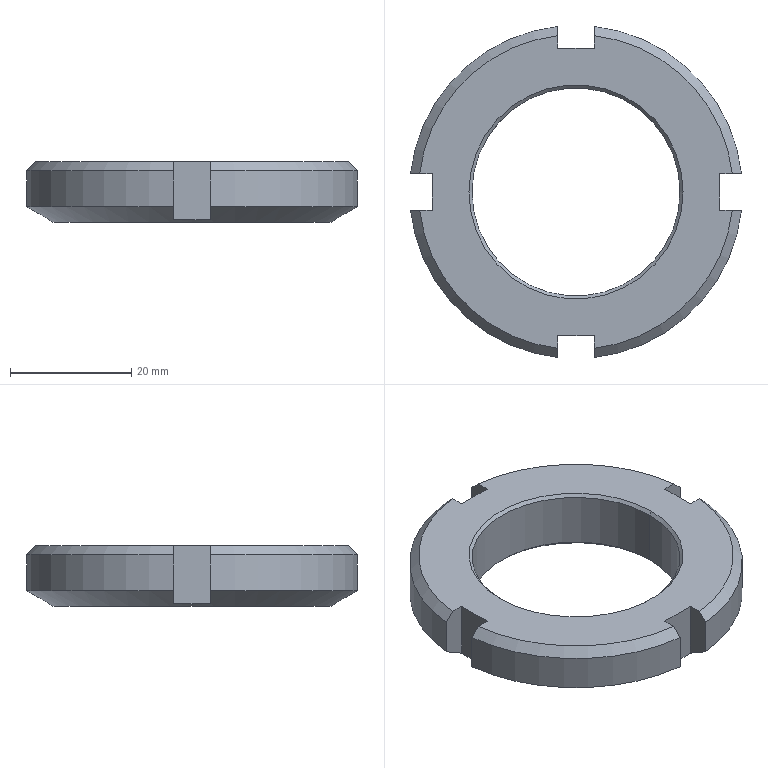Part | SolidWorks | features Chamfer 3, CirPattern 1, Cut 1, Extrusion 1 | 1 solid | 30 faces | box 54.672 x 54.672 x 10 mm | volume 12577 mm3 | plane 14 | cone 10 | cylinder 6 | commonest cylinder face diameters 55 x4 34.376 x2
STEP:
#1=CARTESIAN_POINT('',(-17.188,0.,9.5));
#2=VERTEX_POINT('',#1);
#3=CARTESIAN_POINT('',(17.188,0.,9.5));
#4=VERTEX_POINT('',#3);
#5=CARTESIAN_POINT('',(0.,0.,9.5));
#6=DIRECTION('',(0.,0.,1.));
#7=DIRECTION('',(1.,0.,0.));
#8=AXIS2_PLACEMENT_3D('',#5,#6,#7);
#9=CIRCLE('',#8,17.188);
#10=EDGE_CURVE('',#2,#4,#9,.T.);
#11=ORIENTED_EDGE('',*,*,#10,.F.);
#12=CARTESIAN_POINT('',(-17.688,0.,10.));
#13=VERTEX_POINT('',#12);
#14=CARTESIAN_POINT('',(-17.188,0.,9.5));
#15=DIRECTION('',(-0.7071,0.,0.7071));
#16=VECTOR('',#15,1000.);
#17=LINE('',#14,#16);
#18=EDGE_CURVE('',#2,#13,#17,.T.);
#19=ORIENTED_EDGE('',*,*,#18,.T.);
#20=CARTESIAN_POINT('',(17.688,0.,10.));
#21=VERTEX_POINT('',#20);
#22=CARTESIAN_POINT('',(0.,0.,10.));
#23=DIRECTION('',(0.,0.,-1.));
#24=DIRECTION('',(1.,0.,0.));
#25=AXIS2_PLACEMENT_3D('',#22,#23,#24);
#26=CIRCLE('',#25,17.688);
#27=EDGE_CURVE('',#21,#13,#26,.T.);
#28=ORIENTED_EDGE('',*,*,#27,.F.);
#29=CARTESIAN_POINT('',(17.188,0.,9.5));
#30=DIRECTION('',(0.7071,0.,0.7071));
#31=VECTOR('',#30,1000.);
#32=LINE('',#29,#31);
#33=EDGE_CURVE('',#4,#21,#32,.T.);
#34=ORIENTED_EDGE('',*,*,#33,.F.);
#35=EDGE_LOOP('',(#11,#19,#28,#34));
#36=FACE_OUTER_BOUND('',#35,.T.);
#37=CARTESIAN_POINT('',(0.,0.,9.5));
#38=DIRECTION('',(0.,0.,1.));
#39=DIRECTION('',(1.,0.,0.));
#40=AXIS2_PLACEMENT_3D('',#37,#38,#39);
#41=CONICAL_SURFACE('',#40,17.188,0.7854);
#42=ADVANCED_FACE('',(#36),#41,.F.);
#43=CARTESIAN_POINT('',(17.188,0.,0.5));
#44=VERTEX_POINT('',#43);
#45=CARTESIAN_POINT('',(-17.188,0.,0.5));
#46=VERTEX_POINT('',#45);
#47=CARTESIAN_POINT('',(0.,0.,0.5));
#48=DIRECTION('',(0.,0.,-1.));
#49=DIRECTION('',(1.,0.,0.));
#50=AXIS2_PLACEMENT_3D('',#47,#48,#49);
#51=CIRCLE('',#50,17.188);
#52=EDGE_CURVE('',#44,#46,#51,.T.);
#53=ORIENTED_EDGE('',*,*,#52,.F.);
#54=CARTESIAN_POINT('',(17.688,0.,0.));
#55=VERTEX_POINT('',#54);
#56=CARTESIAN_POINT('',(17.688,0.,0.));
#57=DIRECTION('',(0.7071,0.,-0.7071));
#58=VECTOR('',#57,1000.);
#59=LINE('',#56,#58);
#60=EDGE_CURVE('',#44,#55,#59,.T.);
#61=ORIENTED_EDGE('',*,*,#60,.T.);
#62=CARTESIAN_POINT('',(-17.688,0.,0.));
#63=VERTEX_POINT('',#62);
#64=CARTESIAN_POINT('',(0.,0.,0.));
#65=DIRECTION('',(0.,0.,1.));
#66=DIRECTION('',(1.,0.,0.));
#67=AXIS2_PLACEMENT_3D('',#64,#65,#66);
#68=CIRCLE('',#67,17.688);
#69=EDGE_CURVE('',#63,#55,#68,.T.);
#70=ORIENTED_EDGE('',*,*,#69,.F.);
#71=CARTESIAN_POINT('',(-17.688,0.,0.));
#72=DIRECTION('',(-0.7071,0.,-0.7071));
#73=VECTOR('',#72,1000.);
#74=LINE('',#71,#73);
#75=EDGE_CURVE('',#46,#63,#74,.T.);
#76=ORIENTED_EDGE('',*,*,#75,.F.);
#77=EDGE_LOOP('',(#53,#61,#70,#76));
#78=FACE_OUTER_BOUND('',#77,.T.);
#79=CARTESIAN_POINT('',(0.,0.,0.));
#80=DIRECTION('',(0.,0.,-1.));
#81=DIRECTION('',(-1.,0.,0.));
#82=AXIS2_PLACEMENT_3D('',#79,#80,#81);
#83=CONICAL_SURFACE('',#82,17.688,0.7854);
#84=ADVANCED_FACE('',(#78),#83,.F.);
#85=CARTESIAN_POINT('',(-23.,0.,0.));
#86=VERTEX_POINT('',#85);
#87=CARTESIAN_POINT('',(23.,0.,0.));
#88=VERTEX_POINT('',#87);
#89=CARTESIAN_POINT('',(0.,0.,0.));
#90=DIRECTION('',(0.,0.,-1.));
#91=DIRECTION('',(1.,0.,0.));
#92=AXIS2_PLACEMENT_3D('',#89,#90,#91);
#93=CIRCLE('',#92,23.);
#94=EDGE_CURVE('',#86,#88,#93,.T.);
#95=ORIENTED_EDGE('',*,*,#94,.F.);
#96=CARTESIAN_POINT('',(-23.736,0.,0.4249));
#97=VERTEX_POINT('',#96);
#98=CARTESIAN_POINT('',(-27.5,0.,2.598));
#99=DIRECTION('',(-0.866,0.,0.5));
#100=VECTOR('',#99,1000.);
#101=LINE('',#98,#100);
#102=EDGE_CURVE('',#86,#97,#101,.T.);
#103=ORIENTED_EDGE('',*,*,#102,.T.);
#104=CARTESIAN_POINT('',(-23.736,3.,0.5339));
#105=VERTEX_POINT('',#104);
#106=CARTESIAN_POINT('',(-23.736,3.,0.5339));
#107=CARTESIAN_POINT('',(-23.736,2.004,0.4617));
#108=CARTESIAN_POINT('',(-23.736,1.004,0.4249));
#109=CARTESIAN_POINT('',(-23.736,0.,0.4249));
#110=B_SPLINE_CURVE_WITH_KNOTS('',3,(#106,#107,#108,#109),.UNSPECIFIED.,.F.,.F.,(4,4),(0.008011,0.01101),.UNSPECIFIED.);
#111=EDGE_CURVE('',#105,#97,#110,.T.);
#112=ORIENTED_EDGE('',*,*,#111,.F.);
#113=CARTESIAN_POINT('',(-27.336,3.,2.598));
#114=VERTEX_POINT('',#113);
#115=CARTESIAN_POINT('',(-27.336,3.,2.598));
#116=CARTESIAN_POINT('',(-26.136,3.,1.91));
#117=CARTESIAN_POINT('',(-24.936,3.,1.221));
#118=CARTESIAN_POINT('',(-23.736,3.,0.5339));
#119=B_SPLINE_CURVE_WITH_KNOTS('',3,(#115,#116,#117,#118),.UNSPECIFIED.,.F.,.F.,(4,4),(0.007772,0.01192),.UNSPECIFIED.);
#120=EDGE_CURVE('',#114,#105,#119,.T.);
#121=ORIENTED_EDGE('',*,*,#120,.F.);
#122=CARTESIAN_POINT('',(-3.,27.336,2.598));
#123=VERTEX_POINT('',#122);
#124=CARTESIAN_POINT('',(0.,0.,2.598));
#125=DIRECTION('',(0.,0.,1.));
#126=DIRECTION('',(1.,0.,0.));
#127=AXIS2_PLACEMENT_3D('',#124,#125,#126);
#128=CIRCLE('',#127,27.5);
#129=EDGE_CURVE('',#123,#114,#128,.T.);
#130=ORIENTED_EDGE('',*,*,#129,.F.);
#131=CARTESIAN_POINT('',(-3.,23.736,0.5339));
#132=VERTEX_POINT('',#131);
#133=CARTESIAN_POINT('',(-3.,23.736,0.5339));
#134=CARTESIAN_POINT('',(-3.,24.936,1.221));
#135=CARTESIAN_POINT('',(-3.,26.136,1.91));
#136=CARTESIAN_POINT('',(-3.,27.336,2.598));
#137=B_SPLINE_CURVE_WITH_KNOTS('',3,(#133,#134,#135,#136),.UNSPECIFIED.,.F.,.F.,(4,4),(0.008037,0.01219),.UNSPECIFIED.);
#138=EDGE_CURVE('',#132,#123,#137,.T.);
#139=ORIENTED_EDGE('',*,*,#138,.F.);
#140=CARTESIAN_POINT('',(3.,23.736,0.5339));
#141=VERTEX_POINT('',#140);
#142=CARTESIAN_POINT('',(3.,23.736,0.5339));
#143=CARTESIAN_POINT('',(2.007,23.736,0.462));
#144=CARTESIAN_POINT('',(1.01,23.736,0.4251));
#145=CARTESIAN_POINT('',(-0.9903,23.736,0.4246));
#146=CARTESIAN_POINT('',(-1.998,23.736,0.4613));
#147=CARTESIAN_POINT('',(-3.,23.736,0.5339));
#148=B_SPLINE_CURVE_WITH_KNOTS('',3,(#142,#143,#144,#145,#146,#147),.UNSPECIFIED.,.F.,.F.,(4,2,4),(0.008011,0.011,0.01398),.UNSPECIFIED.);
#149=EDGE_CURVE('',#141,#132,#148,.T.);
#150=ORIENTED_EDGE('',*,*,#149,.F.);
#151=CARTESIAN_POINT('',(3.,27.336,2.598));
#152=VERTEX_POINT('',#151);
#153=CARTESIAN_POINT('',(3.,27.336,2.598));
#154=CARTESIAN_POINT('',(3.,26.136,1.91));
#155=CARTESIAN_POINT('',(3.,24.936,1.221));
#156=CARTESIAN_POINT('',(3.,23.736,0.5339));
#157=B_SPLINE_CURVE_WITH_KNOTS('',3,(#153,#154,#155,#156),.UNSPECIFIED.,.F.,.F.,(4,4),(0.004783,0.008933),.UNSPECIFIED.);
#158=EDGE_CURVE('',#152,#141,#157,.T.);
#159=ORIENTED_EDGE('',*,*,#158,.F.);
#160=CARTESIAN_POINT('',(27.336,3.,2.598));
#161=VERTEX_POINT('',#160);
#162=CARTESIAN_POINT('',(0.,0.,2.598));
#163=DIRECTION('',(0.,0.,1.));
#164=DIRECTION('',(1.,0.,0.));
#165=AXIS2_PLACEMENT_3D('',#162,#163,#164);
#166=CIRCLE('',#165,27.5);
#167=EDGE_CURVE('',#161,#152,#166,.T.);
#168=ORIENTED_EDGE('',*,*,#167,.F.);
#169=CARTESIAN_POINT('',(23.736,3.,0.5339));
#170=VERTEX_POINT('',#169);
#171=CARTESIAN_POINT('',(23.736,3.,0.5339));
#172=CARTESIAN_POINT('',(24.936,3.,1.221));
#173=CARTESIAN_POINT('',(26.136,3.,1.91));
#174=CARTESIAN_POINT('',(27.336,3.,2.598));
#175=B_SPLINE_CURVE_WITH_KNOTS('',3,(#171,#172,#173,#174),.UNSPECIFIED.,.F.,.F.,(4,4),(0.008037,0.01219),.UNSPECIFIED.);
#176=EDGE_CURVE('',#170,#161,#175,.T.);
#177=ORIENTED_EDGE('',*,*,#176,.F.);
#178=CARTESIAN_POINT('',(23.736,0.,0.4249));
#179=VERTEX_POINT('',#178);
#180=CARTESIAN_POINT('',(23.736,0.,0.4249));
#181=CARTESIAN_POINT('',(23.736,1.004,0.4249));
#182=CARTESIAN_POINT('',(23.736,2.004,0.4617));
#183=CARTESIAN_POINT('',(23.736,3.,0.5339));
#184=B_SPLINE_CURVE_WITH_KNOTS('',3,(#180,#181,#182,#183),.UNSPECIFIED.,.F.,.F.,(4,4),(0.01546,0.01847),.UNSPECIFIED.);
#185=EDGE_CURVE('',#179,#170,#184,.T.);
#186=ORIENTED_EDGE('',*,*,#185,.F.);
#187=CARTESIAN_POINT('',(27.5,0.,2.598));
#188=DIRECTION('',(0.866,0.,0.5));
#189=VECTOR('',#188,1000.);
#190=LINE('',#187,#189);
#191=EDGE_CURVE('',#88,#179,#190,.T.);
#192=ORIENTED_EDGE('',*,*,#191,.F.);
#193=EDGE_LOOP('',(#95,#103,#112,#121,#130,#139,#150,#159,#168,#177,#186,#192));
#194=FACE_OUTER_BOUND('',#193,.T.);
#195=CARTESIAN_POINT('',(0.,0.,2.598));
#196=DIRECTION('',(0.,0.,1.));
#197=DIRECTION('',(1.,0.,0.));
#198=AXIS2_PLACEMENT_3D('',#195,#196,#197);
#199=CONICAL_SURFACE('',#198,27.5,1.047);
#200=ADVANCED_FACE('',(#194),#199,.T.);
#201=ORIENTED_EDGE('',*,*,#10,.T.);
#202=CARTESIAN_POINT('',(17.188,0.,10.));
#203=DIRECTION('',(0.,0.,-1.));
#204=VECTOR('',#203,1000.);
#205=LINE('',#202,#204);
#206=EDGE_CURVE('',#4,#44,#205,.T.);
#207=ORIENTED_EDGE('',*,*,#206,.T.);
#208=ORIENTED_EDGE('',*,*,#52,.T.);
#209=CARTESIAN_POINT('',(-17.188,0.,10.));
#210=DIRECTION('',(0.,0.,-1.));
#211=VECTOR('',#210,1000.);
#212=LINE('',#209,#211);
#213=EDGE_CURVE('',#2,#46,#212,.T.);
#214=ORIENTED_EDGE('',*,*,#213,.F.);
#215=EDGE_LOOP('',(#201,#207,#208,#214));
#216=FACE_OUTER_BOUND('',#215,.T.);
#217=CARTESIAN_POINT('',(0.,0.,10.));
#218=DIRECTION('',(0.,0.,-1.));
#219=DIRECTION('',(-1.,0.,0.));
#220=AXIS2_PLACEMENT_3D('',#217,#218,#219);
#221=CYLINDRICAL_SURFACE('',#220,17.188);
#222=ADVANCED_FACE('',(#216),#221,.F.);
#223=CARTESIAN_POINT('',(3.,27.336,8.5));
#224=VERTEX_POINT('',#223);
#225=CARTESIAN_POINT('',(27.336,3.,8.5));
#226=VERTEX_POINT('',#225);
#227=CARTESIAN_POINT('',(0.,0.,8.5));
#228=DIRECTION('',(0.,0.,-1.));
#229=DIRECTION('',(1.,0.,0.));
#230=AXIS2_PLACEMENT_3D('',#227,#228,#229);
#231=CIRCLE('',#230,27.5);
#232=EDGE_CURVE('',#224,#226,#231,.T.);
#233=ORIENTED_EDGE('',*,*,#232,.T.);
#234=CARTESIAN_POINT('',(27.336,3.,0.));
#235=DIRECTION('',(0.,0.,1.));
#236=VECTOR('',#235,1000.);
#237=LINE('',#234,#236);
#238=EDGE_CURVE('',#161,#226,#237,.T.);
#239=ORIENTED_EDGE('',*,*,#238,.F.);
#240=ORIENTED_EDGE('',*,*,#167,.T.);
#241=CARTESIAN_POINT('',(3.,27.336,0.));
#242=DIRECTION('',(0.,0.,1.));
#243=VECTOR('',#242,1000.);
#244=LINE('',#241,#243);
#245=EDGE_CURVE('',#152,#224,#244,.T.);
#246=ORIENTED_EDGE('',*,*,#245,.T.);
#247=EDGE_LOOP('',(#233,#239,#240,#246));
#248=FACE_OUTER_BOUND('',#247,.T.);
#249=CARTESIAN_POINT('',(0.,0.,10.));
#250=DIRECTION('',(0.,0.,-1.));
#251=DIRECTION('',(-1.,0.,0.));
#252=AXIS2_PLACEMENT_3D('',#249,#250,#251);
#253=CYLINDRICAL_SURFACE('',#252,27.5);
#254=ADVANCED_FACE('',(#248),#253,.T.);
#255=CARTESIAN_POINT('',(25.826,3.,10.));
#256=VERTEX_POINT('',#255);
#257=CARTESIAN_POINT('',(27.336,3.,8.5));
#258=CARTESIAN_POINT('',(26.922,3.,8.911));
#259=CARTESIAN_POINT('',(26.508,3.,9.323));
#260=CARTESIAN_POINT('',(26.094,3.,9.734));
#261=CARTESIAN_POINT('',(26.005,3.,9.823));
#262=CARTESIAN_POINT('',(25.916,3.,9.911));
#263=CARTESIAN_POINT('',(25.826,3.,10.));
#264=B_SPLINE_CURVE_WITH_KNOTS('',3,(#257,#258,#259,#260,#261,#262,#263),.UNSPECIFIED.,.F.,.F.,(4,3,4),(0.006071,0.007821,0.008199),.UNSPECIFIED.);
#265=EDGE_CURVE('',#226,#256,#264,.T.);
#266=ORIENTED_EDGE('',*,*,#265,.F.);
#267=ORIENTED_EDGE('',*,*,#232,.F.);
#268=CARTESIAN_POINT('',(3.,25.826,10.));
#269=VERTEX_POINT('',#268);
#270=CARTESIAN_POINT('',(3.,25.826,10.));
#271=CARTESIAN_POINT('',(3.,25.916,9.911));
#272=CARTESIAN_POINT('',(3.,26.005,9.823));
#273=CARTESIAN_POINT('',(3.,26.094,9.734));
#274=CARTESIAN_POINT('',(3.,26.508,9.323));
#275=CARTESIAN_POINT('',(3.,26.922,8.911));
#276=CARTESIAN_POINT('',(3.,27.336,8.5));
#277=B_SPLINE_CURVE_WITH_KNOTS('',3,(#270,#271,#272,#273,#274,#275,#276),.UNSPECIFIED.,.F.,.F.,(4,3,4),(0.007444,0.007821,0.009572),.UNSPECIFIED.);
#278=EDGE_CURVE('',#269,#224,#277,.T.);
#279=ORIENTED_EDGE('',*,*,#278,.F.);
#280=CARTESIAN_POINT('',(0.,0.,10.));
#281=DIRECTION('',(0.,0.,1.));
#282=DIRECTION('',(1.,0.,0.));
#283=AXIS2_PLACEMENT_3D('',#280,#281,#282);
#284=CIRCLE('',#283,26.);
#285=EDGE_CURVE('',#256,#269,#284,.T.);
#286=ORIENTED_EDGE('',*,*,#285,.F.);
#287=EDGE_LOOP('',(#266,#267,#279,#286));
#288=FACE_OUTER_BOUND('',#287,.T.);
#289=CARTESIAN_POINT('',(0.,0.,10.));
#290=DIRECTION('',(0.,0.,-1.));
#291=DIRECTION('',(-1.,0.,0.));
#292=AXIS2_PLACEMENT_3D('',#289,#290,#291);
#293=CONICAL_SURFACE('',#292,26.,0.7854);
#294=ADVANCED_FACE('',(#288),#293,.T.);
#295=CARTESIAN_POINT('',(-27.336,3.,8.5));
#296=VERTEX_POINT('',#295);
#297=CARTESIAN_POINT('',(-3.,27.336,8.5));
#298=VERTEX_POINT('',#297);
#299=CARTESIAN_POINT('',(0.,0.,8.5));
#300=DIRECTION('',(0.,0.,-1.));
#301=DIRECTION('',(1.,0.,0.));
#302=AXIS2_PLACEMENT_3D('',#299,#300,#301);
#303=CIRCLE('',#302,27.5);
#304=EDGE_CURVE('',#296,#298,#303,.T.);
#305=ORIENTED_EDGE('',*,*,#304,.T.);
#306=CARTESIAN_POINT('',(-3.,27.336,0.));
#307=DIRECTION('',(0.,0.,1.));
#308=VECTOR('',#307,1000.);
#309=LINE('',#306,#308);
#310=EDGE_CURVE('',#123,#298,#309,.T.);
#311=ORIENTED_EDGE('',*,*,#310,.F.);
#312=ORIENTED_EDGE('',*,*,#129,.T.);
#313=CARTESIAN_POINT('',(-27.336,3.,0.));
#314=DIRECTION('',(0.,0.,1.));
#315=VECTOR('',#314,1000.);
#316=LINE('',#313,#315);
#317=EDGE_CURVE('',#114,#296,#316,.T.);
#318=ORIENTED_EDGE('',*,*,#317,.T.);
#319=EDGE_LOOP('',(#305,#311,#312,#318));
#320=FACE_OUTER_BOUND('',#319,.T.);
#321=CARTESIAN_POINT('',(0.,0.,10.));
#322=DIRECTION('',(0.,0.,-1.));
#323=DIRECTION('',(-1.,0.,0.));
#324=AXIS2_PLACEMENT_3D('',#321,#322,#323);
#325=CYLINDRICAL_SURFACE('',#324,27.5);
#326=ADVANCED_FACE('',(#320),#325,.T.);
#327=CARTESIAN_POINT('',(-3.,25.826,10.));
#328=VERTEX_POINT('',#327);
#329=CARTESIAN_POINT('',(-3.,27.336,8.5));
#330=CARTESIAN_POINT('',(-3.,26.922,8.911));
#331=CARTESIAN_POINT('',(-3.,26.508,9.323));
#332=CARTESIAN_POINT('',(-3.,26.094,9.734));
#333=CARTESIAN_POINT('',(-3.,26.005,9.823));
#334=CARTESIAN_POINT('',(-3.,25.916,9.911));
#335=CARTESIAN_POINT('',(-3.,25.826,10.));
#336=B_SPLINE_CURVE_WITH_KNOTS('',3,(#329,#330,#331,#332,#333,#334,#335),.UNSPECIFIED.,.F.,.F.,(4,3,4),(0.006071,0.007821,0.008199),.UNSPECIFIED.);
#337=EDGE_CURVE('',#298,#328,#336,.T.);
#338=ORIENTED_EDGE('',*,*,#337,.F.);
#339=ORIENTED_EDGE('',*,*,#304,.F.);
#340=CARTESIAN_POINT('',(-25.826,3.,10.));
#341=VERTEX_POINT('',#340);
#342=CARTESIAN_POINT('',(-25.826,3.,10.));
#343=CARTESIAN_POINT('',(-26.192,3.,9.637));
#344=CARTESIAN_POINT('',(-26.557,3.,9.274));
#345=CARTESIAN_POINT('',(-26.922,3.,8.911));
#346=CARTESIAN_POINT('',(-27.06,3.,8.774));
#347=CARTESIAN_POINT('',(-27.198,3.,8.637));
#348=CARTESIAN_POINT('',(-27.336,3.,8.5));
#349=B_SPLINE_CURVE_WITH_KNOTS('',3,(#342,#343,#344,#345,#346,#347,#348),.UNSPECIFIED.,.F.,.F.,(4,3,4),(0.006277,0.007821,0.008405),.UNSPECIFIED.);
#350=EDGE_CURVE('',#341,#296,#349,.T.);
#351=ORIENTED_EDGE('',*,*,#350,.F.);
#352=CARTESIAN_POINT('',(0.,0.,10.));
#353=DIRECTION('',(0.,0.,1.));
#354=DIRECTION('',(1.,0.,0.));
#355=AXIS2_PLACEMENT_3D('',#352,#353,#354);
#356=CIRCLE('',#355,26.);
#357=EDGE_CURVE('',#328,#341,#356,.T.);
#358=ORIENTED_EDGE('',*,*,#357,.F.);
#359=EDGE_LOOP('',(#338,#339,#351,#358));
#360=FACE_OUTER_BOUND('',#359,.T.);
#361=CARTESIAN_POINT('',(0.,0.,10.));
#362=DIRECTION('',(0.,0.,-1.));
#363=DIRECTION('',(-1.,0.,0.));
#364=AXIS2_PLACEMENT_3D('',#361,#362,#363);
#365=CONICAL_SURFACE('',#364,26.,0.7854);
#366=ADVANCED_FACE('',(#360),#365,.T.);
#367=CARTESIAN_POINT('',(-3.,-27.336,8.5));
#368=VERTEX_POINT('',#367);
#369=CARTESIAN_POINT('',(-27.336,-3.,8.5));
#370=VERTEX_POINT('',#369);
#371=CARTESIAN_POINT('',(0.,0.,8.5));
#372=DIRECTION('',(0.,0.,-1.));
#373=DIRECTION('',(1.,0.,0.));
#374=AXIS2_PLACEMENT_3D('',#371,#372,#373);
#375=CIRCLE('',#374,27.5);
#376=EDGE_CURVE('',#368,#370,#375,.T.);
#377=ORIENTED_EDGE('',*,*,#376,.T.);
#378=CARTESIAN_POINT('',(-27.336,-3.,2.598));
#379=VERTEX_POINT('',#378);
#380=CARTESIAN_POINT('',(-27.336,-3.,0.));
#381=DIRECTION('',(0.,0.,1.));
#382=VECTOR('',#381,1000.);
#383=LINE('',#380,#382);
#384=EDGE_CURVE('',#379,#370,#383,.T.);
#385=ORIENTED_EDGE('',*,*,#384,.F.);
#386=CARTESIAN_POINT('',(-3.,-27.336,2.598));
#387=VERTEX_POINT('',#386);
#388=CARTESIAN_POINT('',(0.,0.,2.598));
#389=DIRECTION('',(0.,0.,1.));
#390=DIRECTION('',(1.,0.,0.));
#391=AXIS2_PLACEMENT_3D('',#388,#389,#390);
#392=CIRCLE('',#391,27.5);
#393=EDGE_CURVE('',#379,#387,#392,.T.);
#394=ORIENTED_EDGE('',*,*,#393,.T.);
#395=CARTESIAN_POINT('',(-3.,-27.336,0.));
#396=DIRECTION('',(0.,0.,1.));
#397=VECTOR('',#396,1000.);
#398=LINE('',#395,#397);
#399=EDGE_CURVE('',#387,#368,#398,.T.);
#400=ORIENTED_EDGE('',*,*,#399,.T.);
#401=EDGE_LOOP('',(#377,#385,#394,#400));
#402=FACE_OUTER_BOUND('',#401,.T.);
#403=CARTESIAN_POINT('',(0.,0.,10.));
#404=DIRECTION('',(0.,0.,-1.));
#405=DIRECTION('',(-1.,0.,0.));
#406=AXIS2_PLACEMENT_3D('',#403,#404,#405);
#407=CYLINDRICAL_SURFACE('',#406,27.5);
#408=ADVANCED_FACE('',(#402),#407,.T.);
#409=CARTESIAN_POINT('',(-25.826,-3.,10.));
#410=VERTEX_POINT('',#409);
#411=CARTESIAN_POINT('',(-27.336,-3.,8.5));
#412=CARTESIAN_POINT('',(-27.198,-3.,8.637));
#413=CARTESIAN_POINT('',(-27.06,-3.,8.774));
#414=CARTESIAN_POINT('',(-26.922,-3.,8.911));
#415=CARTESIAN_POINT('',(-26.557,-3.,9.274));
#416=CARTESIAN_POINT('',(-26.192,-3.,9.637));
#417=CARTESIAN_POINT('',(-25.826,-3.,10.));
#418=B_SPLINE_CURVE_WITH_KNOTS('',3,(#411,#412,#413,#414,#415,#416,#417),.UNSPECIFIED.,.F.,.F.,(4,3,4),(0.007238,0.007821,0.009366),.UNSPECIFIED.);
#419=EDGE_CURVE('',#370,#410,#418,.T.);
#420=ORIENTED_EDGE('',*,*,#419,.F.);
#421=ORIENTED_EDGE('',*,*,#376,.F.);
#422=CARTESIAN_POINT('',(-3.,-25.826,10.));
#423=VERTEX_POINT('',#422);
#424=CARTESIAN_POINT('',(-3.,-25.826,10.));
#425=CARTESIAN_POINT('',(-3.,-26.192,9.637));
#426=CARTESIAN_POINT('',(-3.,-26.557,9.274));
#427=CARTESIAN_POINT('',(-3.,-26.922,8.911));
#428=CARTESIAN_POINT('',(-3.,-27.06,8.774));
#429=CARTESIAN_POINT('',(-3.,-27.198,8.637));
#430=CARTESIAN_POINT('',(-3.,-27.336,8.5));
#431=B_SPLINE_CURVE_WITH_KNOTS('',3,(#424,#425,#426,#427,#428,#429,#430),.UNSPECIFIED.,.F.,.F.,(4,3,4),(0.006277,0.007821,0.008405),.UNSPECIFIED.);
#432=EDGE_CURVE('',#423,#368,#431,.T.);
#433=ORIENTED_EDGE('',*,*,#432,.F.);
#434=CARTESIAN_POINT('',(0.,0.,10.));
#435=DIRECTION('',(0.,0.,1.));
#436=DIRECTION('',(1.,0.,0.));
#437=AXIS2_PLACEMENT_3D('',#434,#435,#436);
#438=CIRCLE('',#437,26.);
#439=EDGE_CURVE('',#410,#423,#438,.T.);
#440=ORIENTED_EDGE('',*,*,#439,.F.);
#441=EDGE_LOOP('',(#420,#421,#433,#440));
#442=FACE_OUTER_BOUND('',#441,.T.);
#443=CARTESIAN_POINT('',(0.,0.,10.));
#444=DIRECTION('',(0.,0.,-1.));
#445=DIRECTION('',(-1.,0.,0.));
#446=AXIS2_PLACEMENT_3D('',#443,#444,#445);
#447=CONICAL_SURFACE('',#446,26.,0.7854);
#448=ADVANCED_FACE('',(#442),#447,.T.);
#449=ORIENTED_EDGE('',*,*,#27,.T.);
#450=CARTESIAN_POINT('',(0.,0.,10.));
#451=DIRECTION('',(0.,0.,-1.));
#452=DIRECTION('',(1.,0.,0.));
#453=AXIS2_PLACEMENT_3D('',#450,#451,#452);
#454=CIRCLE('',#453,17.688);
#455=EDGE_CURVE('',#13,#21,#454,.T.);
#456=ORIENTED_EDGE('',*,*,#455,.T.);
#457=EDGE_LOOP('',(#449,#456));
#458=FACE_BOUND('',#457,.T.);
#459=CARTESIAN_POINT('',(23.736,3.,10.));
#460=VERTEX_POINT('',#459);
#461=CARTESIAN_POINT('',(23.736,3.,10.));
#462=DIRECTION('',(-1.,0.,0.));
#463=VECTOR('',#462,1000.);
#464=LINE('',#461,#463);
#465=EDGE_CURVE('',#256,#460,#464,.T.);
#466=ORIENTED_EDGE('',*,*,#465,.F.);
#467=ORIENTED_EDGE('',*,*,#285,.T.);
#468=CARTESIAN_POINT('',(3.,23.736,10.));
#469=VERTEX_POINT('',#468);
#470=CARTESIAN_POINT('',(3.,23.736,10.));
#471=DIRECTION('',(0.,1.,0.));
#472=VECTOR('',#471,1000.);
#473=LINE('',#470,#472);
#474=EDGE_CURVE('',#469,#269,#473,.T.);
#475=ORIENTED_EDGE('',*,*,#474,.F.);
#476=CARTESIAN_POINT('',(-3.,23.736,10.));
#477=VERTEX_POINT('',#476);
#478=CARTESIAN_POINT('',(3.,23.736,10.));
#479=DIRECTION('',(1.,0.,0.));
#480=VECTOR('',#479,1000.);
#481=LINE('',#478,#480);
#482=EDGE_CURVE('',#477,#469,#481,.T.);
#483=ORIENTED_EDGE('',*,*,#482,.F.);
#484=CARTESIAN_POINT('',(-3.,23.736,10.));
#485=DIRECTION('',(0.,-1.,0.));
#486=VECTOR('',#485,1000.);
#487=LINE('',#484,#486);
#488=EDGE_CURVE('',#328,#477,#487,.T.);
#489=ORIENTED_EDGE('',*,*,#488,.F.);
#490=ORIENTED_EDGE('',*,*,#357,.T.);
#491=CARTESIAN_POINT('',(-23.736,3.,10.));
#492=VERTEX_POINT('',#491);
#493=CARTESIAN_POINT('',(-23.736,3.,10.));
#494=DIRECTION('',(-1.,0.,0.));
#495=VECTOR('',#494,1000.);
#496=LINE('',#493,#495);
#497=EDGE_CURVE('',#492,#341,#496,.T.);
#498=ORIENTED_EDGE('',*,*,#497,.F.);
#499=CARTESIAN_POINT('',(-23.736,-3.,10.));
#500=VERTEX_POINT('',#499);
#501=CARTESIAN_POINT('',(-23.736,3.,10.));
#502=DIRECTION('',(0.,1.,0.));
#503=VECTOR('',#502,1000.);
#504=LINE('',#501,#503);
#505=EDGE_CURVE('',#500,#492,#504,.T.);
#506=ORIENTED_EDGE('',*,*,#505,.F.);
#507=CARTESIAN_POINT('',(-23.736,-3.,10.));
#508=DIRECTION('',(1.,0.,0.));
#509=VECTOR('',#508,1000.);
#510=LINE('',#507,#509);
#511=EDGE_CURVE('',#410,#500,#510,.T.);
#512=ORIENTED_EDGE('',*,*,#511,.F.);
#513=ORIENTED_EDGE('',*,*,#439,.T.);
#514=CARTESIAN_POINT('',(-3.,-23.736,10.));
#515=VERTEX_POINT('',#514);
#516=CARTESIAN_POINT('',(-3.,-23.736,10.));
#517=DIRECTION('',(0.,-1.,0.));
#518=VECTOR('',#517,1000.);
#519=LINE('',#516,#518);
#520=EDGE_CURVE('',#515,#423,#519,.T.);
#521=ORIENTED_EDGE('',*,*,#520,.F.);
#522=CARTESIAN_POINT('',(3.,-23.736,10.));
#523=VERTEX_POINT('',#522);
#524=CARTESIAN_POINT('',(-3.,-23.736,10.));
#525=DIRECTION('',(-1.,0.,0.));
#526=VECTOR('',#525,1000.);
#527=LINE('',#524,#526);
#528=EDGE_CURVE('',#523,#515,#527,.T.);
#529=ORIENTED_EDGE('',*,*,#528,.F.);
#530=CARTESIAN_POINT('',(3.,-25.826,10.));
#531=VERTEX_POINT('',#530);
#532=CARTESIAN_POINT('',(3.,-23.736,10.));
#533=DIRECTION('',(0.,1.,0.));
#534=VECTOR('',#533,1000.);
#535=LINE('',#532,#534);
#536=EDGE_CURVE('',#531,#523,#535,.T.);
#537=ORIENTED_EDGE('',*,*,#536,.F.);
#538=CARTESIAN_POINT('',(25.826,-3.,10.));
#539=VERTEX_POINT('',#538);
#540=CARTESIAN_POINT('',(0.,0.,10.));
#541=DIRECTION('',(0.,0.,1.));
#542=DIRECTION('',(1.,0.,0.));
#543=AXIS2_PLACEMENT_3D('',#540,#541,#542);
#544=CIRCLE('',#543,26.);
#545=EDGE_CURVE('',#531,#539,#544,.T.);
#546=ORIENTED_EDGE('',*,*,#545,.T.);
#547=CARTESIAN_POINT('',(23.736,-3.,10.));
#548=VERTEX_POINT('',#547);
#549=CARTESIAN_POINT('',(23.736,-3.,10.));
#550=DIRECTION('',(1.,0.,0.));
#551=VECTOR('',#550,1000.);
#552=LINE('',#549,#551);
#553=EDGE_CURVE('',#548,#539,#552,.T.);
#554=ORIENTED_EDGE('',*,*,#553,.F.);
#555=CARTESIAN_POINT('',(23.736,-3.,10.));
#556=DIRECTION('',(0.,-1.,0.));
#557=VECTOR('',#556,1000.);
#558=LINE('',#555,#557);
#559=EDGE_CURVE('',#460,#548,#558,.T.);
#560=ORIENTED_EDGE('',*,*,#559,.F.);
#561=EDGE_LOOP('',(#466,#467,#475,#483,#489,#490,#498,#506,#512,#513,#521,#529,#537,#546,#554,#560));
#562=FACE_OUTER_BOUND('',#561,.T.);
#563=CARTESIAN_POINT('',(0.,0.,10.));
#564=DIRECTION('',(0.,0.,1.));
#565=DIRECTION('',(1.,0.,0.));
#566=AXIS2_PLACEMENT_3D('',#563,#564,#565);
#567=PLANE('',#566);
#568=ADVANCED_FACE('',(#458,#562),#567,.T.);
#569=ORIENTED_EDGE('',*,*,#69,.T.);
#570=CARTESIAN_POINT('',(0.,0.,0.));
#571=DIRECTION('',(0.,0.,1.));
#572=DIRECTION('',(1.,0.,0.));
#573=AXIS2_PLACEMENT_3D('',#570,#571,#572);
#574=CIRCLE('',#573,17.688);
#575=EDGE_CURVE('',#55,#63,#574,.T.);
#576=ORIENTED_EDGE('',*,*,#575,.T.);
#577=EDGE_LOOP('',(#569,#576));
#578=FACE_BOUND('',#577,.T.);
#579=CARTESIAN_POINT('',(0.,0.,0.));
#580=DIRECTION('',(0.,0.,-1.));
#581=DIRECTION('',(1.,0.,0.));
#582=AXIS2_PLACEMENT_3D('',#579,#580,#581);
#583=CIRCLE('',#582,23.);
#584=EDGE_CURVE('',#88,#86,#583,.T.);
#585=ORIENTED_EDGE('',*,*,#584,.T.);
#586=ORIENTED_EDGE('',*,*,#94,.T.);
#587=EDGE_LOOP('',(#585,#586));
#588=FACE_OUTER_BOUND('',#587,.T.);
#589=CARTESIAN_POINT('',(0.,0.,0.));
#590=DIRECTION('',(0.,0.,1.));
#591=DIRECTION('',(1.,0.,0.));
#592=AXIS2_PLACEMENT_3D('',#589,#590,#591);
#593=PLANE('',#592);
#594=ADVANCED_FACE('',(#578,#588),#593,.F.);
#595=CARTESIAN_POINT('',(3.,-27.336,2.598));
#596=VERTEX_POINT('',#595);
#597=CARTESIAN_POINT('',(27.336,-3.,2.598));
#598=VERTEX_POINT('',#597);
#599=CARTESIAN_POINT('',(0.,0.,2.598));
#600=DIRECTION('',(0.,0.,1.));
#601=DIRECTION('',(1.,0.,0.));
#602=AXIS2_PLACEMENT_3D('',#599,#600,#601);
#603=CIRCLE('',#602,27.5);
#604=EDGE_CURVE('',#596,#598,#603,.T.);
#605=ORIENTED_EDGE('',*,*,#604,.T.);
#606=CARTESIAN_POINT('',(27.336,-3.,8.5));
#607=VERTEX_POINT('',#606);
#608=CARTESIAN_POINT('',(27.336,-3.,0.));
#609=DIRECTION('',(0.,0.,1.));
#610=VECTOR('',#609,1000.);
#611=LINE('',#608,#610);
#612=EDGE_CURVE('',#598,#607,#611,.T.);
#613=ORIENTED_EDGE('',*,*,#612,.T.);
#614=CARTESIAN_POINT('',(3.,-27.336,8.5));
#615=VERTEX_POINT('',#614);
#616=CARTESIAN_POINT('',(0.,0.,8.5));
#617=DIRECTION('',(0.,0.,-1.));
#618=DIRECTION('',(1.,0.,0.));
#619=AXIS2_PLACEMENT_3D('',#616,#617,#618);
#620=CIRCLE('',#619,27.5);
#621=EDGE_CURVE('',#607,#615,#620,.T.);
#622=ORIENTED_EDGE('',*,*,#621,.T.);
#623=CARTESIAN_POINT('',(3.,-27.336,0.));
#624=DIRECTION('',(0.,0.,1.));
#625=VECTOR('',#624,1000.);
#626=LINE('',#623,#625);
#627=EDGE_CURVE('',#596,#615,#626,.T.);
#628=ORIENTED_EDGE('',*,*,#627,.F.);
#629=EDGE_LOOP('',(#605,#613,#622,#628));
#630=FACE_OUTER_BOUND('',#629,.T.);
#631=CARTESIAN_POINT('',(0.,0.,10.));
#632=DIRECTION('',(0.,0.,-1.));
#633=DIRECTION('',(-1.,0.,0.));
#634=AXIS2_PLACEMENT_3D('',#631,#632,#633);
#635=CYLINDRICAL_SURFACE('',#634,27.5);
#636=ADVANCED_FACE('',(#630),#635,.T.);
#637=ORIENTED_EDGE('',*,*,#206,.F.);
#638=CARTESIAN_POINT('',(0.,0.,9.5));
#639=DIRECTION('',(0.,0.,1.));
#640=DIRECTION('',(1.,0.,0.));
#641=AXIS2_PLACEMENT_3D('',#638,#639,#640);
#642=CIRCLE('',#641,17.188);
#643=EDGE_CURVE('',#4,#2,#642,.T.);
#644=ORIENTED_EDGE('',*,*,#643,.T.);
#645=ORIENTED_EDGE('',*,*,#213,.T.);
#646=CARTESIAN_POINT('',(0.,0.,0.5));
#647=DIRECTION('',(0.,0.,-1.));
#648=DIRECTION('',(1.,0.,0.));
#649=AXIS2_PLACEMENT_3D('',#646,#647,#648);
#650=CIRCLE('',#649,17.188);
#651=EDGE_CURVE('',#46,#44,#650,.T.);
#652=ORIENTED_EDGE('',*,*,#651,.T.);
#653=EDGE_LOOP('',(#637,#644,#645,#652));
#654=FACE_OUTER_BOUND('',#653,.T.);
#655=CARTESIAN_POINT('',(0.,0.,10.));
#656=DIRECTION('',(0.,0.,-1.));
#657=DIRECTION('',(-1.,0.,0.));
#658=AXIS2_PLACEMENT_3D('',#655,#656,#657);
#659=CYLINDRICAL_SURFACE('',#658,17.188);
#660=ADVANCED_FACE('',(#654),#659,.F.);
#661=CARTESIAN_POINT('',(25.826,-3.,10.));
#662=CARTESIAN_POINT('',(25.916,-3.,9.911));
#663=CARTESIAN_POINT('',(26.005,-3.,9.823));
#664=CARTESIAN_POINT('',(26.094,-3.,9.734));
#665=CARTESIAN_POINT('',(26.508,-3.,9.323));
#666=CARTESIAN_POINT('',(26.922,-3.,8.911));
#667=CARTESIAN_POINT('',(27.336,-3.,8.5));
#668=B_SPLINE_CURVE_WITH_KNOTS('',3,(#661,#662,#663,#664,#665,#666,#667),.UNSPECIFIED.,.F.,.F.,(4,3,4),(0.007444,0.007821,0.009572),.UNSPECIFIED.);
#669=EDGE_CURVE('',#539,#607,#668,.T.);
#670=ORIENTED_EDGE('',*,*,#669,.F.);
#671=ORIENTED_EDGE('',*,*,#545,.F.);
#672=CARTESIAN_POINT('',(3.,-27.336,8.5));
#673=CARTESIAN_POINT('',(3.,-27.198,8.637));
#674=CARTESIAN_POINT('',(3.,-27.06,8.774));
#675=CARTESIAN_POINT('',(3.,-26.922,8.911));
#676=CARTESIAN_POINT('',(3.,-26.557,9.274));
#677=CARTESIAN_POINT('',(3.,-26.192,9.637));
#678=CARTESIAN_POINT('',(3.,-25.826,10.));
#679=B_SPLINE_CURVE_WITH_KNOTS('',3,(#672,#673,#674,#675,#676,#677,#678),.UNSPECIFIED.,.F.,.F.,(4,3,4),(0.007238,0.007821,0.009366),.UNSPECIFIED.);
#680=EDGE_CURVE('',#615,#531,#679,.T.);
#681=ORIENTED_EDGE('',*,*,#680,.F.);
#682=ORIENTED_EDGE('',*,*,#621,.F.);
#683=EDGE_LOOP('',(#670,#671,#681,#682));
#684=FACE_OUTER_BOUND('',#683,.T.);
#685=CARTESIAN_POINT('',(0.,0.,10.));
#686=DIRECTION('',(0.,0.,-1.));
#687=DIRECTION('',(-1.,0.,0.));
#688=AXIS2_PLACEMENT_3D('',#685,#686,#687);
#689=CONICAL_SURFACE('',#688,26.,0.7854);
#690=ADVANCED_FACE('',(#684),#689,.T.);
#691=ORIENTED_EDGE('',*,*,#102,.F.);
#692=ORIENTED_EDGE('',*,*,#584,.F.);
#693=ORIENTED_EDGE('',*,*,#191,.T.);
#694=CARTESIAN_POINT('',(23.736,-3.,0.5339));
#695=VERTEX_POINT('',#694);
#696=CARTESIAN_POINT('',(23.736,-3.,0.5339));
#697=CARTESIAN_POINT('',(23.736,-2.001,0.4616));
#698=CARTESIAN_POINT('',(23.736,-0.997,0.4249));
#699=CARTESIAN_POINT('',(23.736,0.,0.4249));
#700=B_SPLINE_CURVE_WITH_KNOTS('',3,(#696,#697,#698,#699),.UNSPECIFIED.,.F.,.F.,(4,4),(0.01248,0.01546),.UNSPECIFIED.);
#701=EDGE_CURVE('',#695,#179,#700,.T.);
#702=ORIENTED_EDGE('',*,*,#701,.F.);
#703=CARTESIAN_POINT('',(27.336,-3.,2.598));
#704=CARTESIAN_POINT('',(26.136,-3.,1.91));
#705=CARTESIAN_POINT('',(24.936,-3.,1.221));
#706=CARTESIAN_POINT('',(23.736,-3.,0.5339));
#707=B_SPLINE_CURVE_WITH_KNOTS('',3,(#703,#704,#705,#706),.UNSPECIFIED.,.F.,.F.,(4,4),(0.004783,0.008933),.UNSPECIFIED.);
#708=EDGE_CURVE('',#598,#695,#707,.T.);
#709=ORIENTED_EDGE('',*,*,#708,.F.);
#710=ORIENTED_EDGE('',*,*,#604,.F.);
#711=CARTESIAN_POINT('',(3.,-23.736,0.5339));
#712=VERTEX_POINT('',#711);
#713=CARTESIAN_POINT('',(3.,-23.736,0.5339));
#714=CARTESIAN_POINT('',(3.,-24.936,1.221));
#715=CARTESIAN_POINT('',(3.,-26.136,1.91));
#716=CARTESIAN_POINT('',(3.,-27.336,2.598));
#717=B_SPLINE_CURVE_WITH_KNOTS('',3,(#713,#714,#715,#716),.UNSPECIFIED.,.F.,.F.,(4,4),(0.005049,0.009199),.UNSPECIFIED.);
#718=EDGE_CURVE('',#712,#596,#717,.T.);
#719=ORIENTED_EDGE('',*,*,#718,.F.);
#720=CARTESIAN_POINT('',(-3.,-23.736,0.5339));
#721=VERTEX_POINT('',#720);
#722=CARTESIAN_POINT('',(-3.,-23.736,0.5339));
#723=CARTESIAN_POINT('',(-1.998,-23.736,0.4613));
#724=CARTESIAN_POINT('',(-0.9903,-23.736,0.4246));
#725=CARTESIAN_POINT('',(1.01,-23.736,0.4251));
#726=CARTESIAN_POINT('',(2.007,-23.736,0.462));
#727=CARTESIAN_POINT('',(3.,-23.736,0.5339));
#728=B_SPLINE_CURVE_WITH_KNOTS('',3,(#722,#723,#724,#725,#726,#727),.UNSPECIFIED.,.F.,.F.,(4,2,4),(0.01248,0.01547,0.01847),.UNSPECIFIED.);
#729=EDGE_CURVE('',#721,#712,#728,.T.);
#730=ORIENTED_EDGE('',*,*,#729,.F.);
#731=CARTESIAN_POINT('',(-3.,-27.336,2.598));
#732=CARTESIAN_POINT('',(-3.,-26.136,1.91));
#733=CARTESIAN_POINT('',(-3.,-24.936,1.221));
#734=CARTESIAN_POINT('',(-3.,-23.736,0.5339));
#735=B_SPLINE_CURVE_WITH_KNOTS('',3,(#731,#732,#733,#734),.UNSPECIFIED.,.F.,.F.,(4,4),(0.007772,0.01192),.UNSPECIFIED.);
#736=EDGE_CURVE('',#387,#721,#735,.T.);
#737=ORIENTED_EDGE('',*,*,#736,.F.);
#738=ORIENTED_EDGE('',*,*,#393,.F.);
#739=CARTESIAN_POINT('',(-23.736,-3.,0.5339));
#740=VERTEX_POINT('',#739);
#741=CARTESIAN_POINT('',(-23.736,-3.,0.5339));
#742=CARTESIAN_POINT('',(-24.936,-3.,1.221));
#743=CARTESIAN_POINT('',(-26.136,-3.,1.91));
#744=CARTESIAN_POINT('',(-27.336,-3.,2.598));
#745=B_SPLINE_CURVE_WITH_KNOTS('',3,(#741,#742,#743,#744),.UNSPECIFIED.,.F.,.F.,(4,4),(0.005049,0.009199),.UNSPECIFIED.);
#746=EDGE_CURVE('',#740,#379,#745,.T.);
#747=ORIENTED_EDGE('',*,*,#746,.F.);
#748=CARTESIAN_POINT('',(-23.736,0.,0.4249));
#749=CARTESIAN_POINT('',(-23.736,-0.997,0.4249));
#750=CARTESIAN_POINT('',(-23.736,-2.001,0.4616));
#751=CARTESIAN_POINT('',(-23.736,-3.,0.5339));
#752=B_SPLINE_CURVE_WITH_KNOTS('',3,(#748,#749,#750,#751),.UNSPECIFIED.,.F.,.F.,(4,4),(0.01101,0.01398),.UNSPECIFIED.);
#753=EDGE_CURVE('',#97,#740,#752,.T.);
#754=ORIENTED_EDGE('',*,*,#753,.F.);
#755=EDGE_LOOP('',(#691,#692,#693,#702,#709,#710,#719,#730,#737,#738,#747,#754));
#756=FACE_OUTER_BOUND('',#755,.T.);
#757=CARTESIAN_POINT('',(0.,0.,2.598));
#758=DIRECTION('',(0.,0.,1.));
#759=DIRECTION('',(1.,0.,0.));
#760=AXIS2_PLACEMENT_3D('',#757,#758,#759);
#761=CONICAL_SURFACE('',#760,27.5,1.047);
#762=ADVANCED_FACE('',(#756),#761,.T.);
#763=ORIENTED_EDGE('',*,*,#729,.T.);
#764=CARTESIAN_POINT('',(3.,-23.736,0.));
#765=DIRECTION('',(0.,0.,1.));
#766=VECTOR('',#765,1000.);
#767=LINE('',#764,#766);
#768=EDGE_CURVE('',#712,#523,#767,.T.);
#769=ORIENTED_EDGE('',*,*,#768,.T.);
#770=ORIENTED_EDGE('',*,*,#528,.T.);
#771=CARTESIAN_POINT('',(-3.,-23.736,0.));
#772=DIRECTION('',(0.,0.,1.));
#773=VECTOR('',#772,1000.);
#774=LINE('',#771,#773);
#775=EDGE_CURVE('',#721,#515,#774,.T.);
#776=ORIENTED_EDGE('',*,*,#775,.F.);
#777=EDGE_LOOP('',(#763,#769,#770,#776));
#778=FACE_OUTER_BOUND('',#777,.T.);
#779=CARTESIAN_POINT('',(-3.,-23.736,0.));
#780=DIRECTION('',(0.,1.,0.));
#781=DIRECTION('',(0.,0.,1.));
#782=AXIS2_PLACEMENT_3D('',#779,#780,#781);
#783=PLANE('',#782);
#784=ADVANCED_FACE('',(#778),#783,.F.);
#785=ORIENTED_EDGE('',*,*,#680,.T.);
#786=ORIENTED_EDGE('',*,*,#536,.T.);
#787=ORIENTED_EDGE('',*,*,#768,.F.);
#788=ORIENTED_EDGE('',*,*,#718,.T.);
#789=ORIENTED_EDGE('',*,*,#627,.T.);
#790=EDGE_LOOP('',(#785,#786,#787,#788,#789));
#791=FACE_OUTER_BOUND('',#790,.T.);
#792=CARTESIAN_POINT('',(3.,-23.736,0.));
#793=DIRECTION('',(1.,0.,0.));
#794=DIRECTION('',(0.,1.,0.));
#795=AXIS2_PLACEMENT_3D('',#792,#793,#794);
#796=PLANE('',#795);
#797=ADVANCED_FACE('',(#791),#796,.F.);
#798=ORIENTED_EDGE('',*,*,#432,.T.);
#799=ORIENTED_EDGE('',*,*,#399,.F.);
#800=ORIENTED_EDGE('',*,*,#736,.T.);
#801=ORIENTED_EDGE('',*,*,#775,.T.);
#802=ORIENTED_EDGE('',*,*,#520,.T.);
#803=EDGE_LOOP('',(#798,#799,#800,#801,#802));
#804=FACE_OUTER_BOUND('',#803,.T.);
#805=CARTESIAN_POINT('',(-3.,-23.736,0.));
#806=DIRECTION('',(-1.,0.,0.));
#807=DIRECTION('',(0.,-1.,0.));
#808=AXIS2_PLACEMENT_3D('',#805,#806,#807);
#809=PLANE('',#808);
#810=ADVANCED_FACE('',(#804),#809,.F.);
#811=ORIENTED_EDGE('',*,*,#111,.T.);
#812=ORIENTED_EDGE('',*,*,#753,.T.);
#813=CARTESIAN_POINT('',(-23.736,-3.,0.));
#814=DIRECTION('',(0.,0.,1.));
#815=VECTOR('',#814,1000.);
#816=LINE('',#813,#815);
#817=EDGE_CURVE('',#740,#500,#816,.T.);
#818=ORIENTED_EDGE('',*,*,#817,.T.);
#819=ORIENTED_EDGE('',*,*,#505,.T.);
#820=CARTESIAN_POINT('',(-23.736,3.,0.));
#821=DIRECTION('',(0.,0.,1.));
#822=VECTOR('',#821,1000.);
#823=LINE('',#820,#822);
#824=EDGE_CURVE('',#105,#492,#823,.T.);
#825=ORIENTED_EDGE('',*,*,#824,.F.);
#826=EDGE_LOOP('',(#811,#812,#818,#819,#825));
#827=FACE_OUTER_BOUND('',#826,.T.);
#828=CARTESIAN_POINT('',(-23.736,3.,0.));
#829=DIRECTION('',(1.,0.,0.));
#830=DIRECTION('',(0.,1.,0.));
#831=AXIS2_PLACEMENT_3D('',#828,#829,#830);
#832=PLANE('',#831);
#833=ADVANCED_FACE('',(#827),#832,.F.);
#834=ORIENTED_EDGE('',*,*,#419,.T.);
#835=ORIENTED_EDGE('',*,*,#511,.T.);
#836=ORIENTED_EDGE('',*,*,#817,.F.);
#837=ORIENTED_EDGE('',*,*,#746,.T.);
#838=ORIENTED_EDGE('',*,*,#384,.T.);
#839=EDGE_LOOP('',(#834,#835,#836,#837,#838));
#840=FACE_OUTER_BOUND('',#839,.T.);
#841=CARTESIAN_POINT('',(-23.736,-3.,0.));
#842=DIRECTION('',(0.,-1.,0.));
#843=DIRECTION('',(1.,0.,0.));
#844=AXIS2_PLACEMENT_3D('',#841,#842,#843);
#845=PLANE('',#844);
#846=ADVANCED_FACE('',(#840),#845,.F.);
#847=ORIENTED_EDGE('',*,*,#350,.T.);
#848=ORIENTED_EDGE('',*,*,#317,.F.);
#849=ORIENTED_EDGE('',*,*,#120,.T.);
#850=ORIENTED_EDGE('',*,*,#824,.T.);
#851=ORIENTED_EDGE('',*,*,#497,.T.);
#852=EDGE_LOOP('',(#847,#848,#849,#850,#851));
#853=FACE_OUTER_BOUND('',#852,.T.);
#854=CARTESIAN_POINT('',(-23.736,3.,0.));
#855=DIRECTION('',(0.,1.,0.));
#856=DIRECTION('',(-1.,0.,0.));
#857=AXIS2_PLACEMENT_3D('',#854,#855,#856);
#858=PLANE('',#857);
#859=ADVANCED_FACE('',(#853),#858,.F.);
#860=ORIENTED_EDGE('',*,*,#149,.T.);
#861=CARTESIAN_POINT('',(-3.,23.736,0.));
#862=DIRECTION('',(0.,0.,1.));
#863=VECTOR('',#862,1000.);
#864=LINE('',#861,#863);
#865=EDGE_CURVE('',#132,#477,#864,.T.);
#866=ORIENTED_EDGE('',*,*,#865,.T.);
#867=ORIENTED_EDGE('',*,*,#482,.T.);
#868=CARTESIAN_POINT('',(3.,23.736,0.));
#869=DIRECTION('',(0.,0.,1.));
#870=VECTOR('',#869,1000.);
#871=LINE('',#868,#870);
#872=EDGE_CURVE('',#141,#469,#871,.T.);
#873=ORIENTED_EDGE('',*,*,#872,.F.);
#874=EDGE_LOOP('',(#860,#866,#867,#873));
#875=FACE_OUTER_BOUND('',#874,.T.);
#876=CARTESIAN_POINT('',(3.,23.736,0.));
#877=DIRECTION('',(0.,-1.,0.));
#878=DIRECTION('',(1.,0.,0.));
#879=AXIS2_PLACEMENT_3D('',#876,#877,#878);
#880=PLANE('',#879);
#881=ADVANCED_FACE('',(#875),#880,.F.);
#882=ORIENTED_EDGE('',*,*,#337,.T.);
#883=ORIENTED_EDGE('',*,*,#488,.T.);
#884=ORIENTED_EDGE('',*,*,#865,.F.);
#885=ORIENTED_EDGE('',*,*,#138,.T.);
#886=ORIENTED_EDGE('',*,*,#310,.T.);
#887=EDGE_LOOP('',(#882,#883,#884,#885,#886));
#888=FACE_OUTER_BOUND('',#887,.T.);
#889=CARTESIAN_POINT('',(-3.,23.736,0.));
#890=DIRECTION('',(-1.,0.,0.));
#891=DIRECTION('',(0.,-1.,0.));
#892=AXIS2_PLACEMENT_3D('',#889,#890,#891);
#893=PLANE('',#892);
#894=ADVANCED_FACE('',(#888),#893,.F.);
#895=ORIENTED_EDGE('',*,*,#278,.T.);
#896=ORIENTED_EDGE('',*,*,#245,.F.);
#897=ORIENTED_EDGE('',*,*,#158,.T.);
#898=ORIENTED_EDGE('',*,*,#872,.T.);
#899=ORIENTED_EDGE('',*,*,#474,.T.);
#900=EDGE_LOOP('',(#895,#896,#897,#898,#899));
#901=FACE_OUTER_BOUND('',#900,.T.);
#902=CARTESIAN_POINT('',(3.,23.736,0.));
#903=DIRECTION('',(1.,0.,0.));
#904=DIRECTION('',(0.,1.,0.));
#905=AXIS2_PLACEMENT_3D('',#902,#903,#904);
#906=PLANE('',#905);
#907=ADVANCED_FACE('',(#901),#906,.F.);
#908=ORIENTED_EDGE('',*,*,#701,.T.);
#909=ORIENTED_EDGE('',*,*,#185,.T.);
#910=CARTESIAN_POINT('',(23.736,3.,0.));
#911=DIRECTION('',(0.,0.,1.));
#912=VECTOR('',#911,1000.);
#913=LINE('',#910,#912);
#914=EDGE_CURVE('',#170,#460,#913,.T.);
#915=ORIENTED_EDGE('',*,*,#914,.T.);
#916=ORIENTED_EDGE('',*,*,#559,.T.);
#917=CARTESIAN_POINT('',(23.736,-3.,0.));
#918=DIRECTION('',(0.,0.,1.));
#919=VECTOR('',#918,1000.);
#920=LINE('',#917,#919);
#921=EDGE_CURVE('',#695,#548,#920,.T.);
#922=ORIENTED_EDGE('',*,*,#921,.F.);
#923=EDGE_LOOP('',(#908,#909,#915,#916,#922));
#924=FACE_OUTER_BOUND('',#923,.T.);
#925=CARTESIAN_POINT('',(23.736,-3.,0.));
#926=DIRECTION('',(-1.,0.,0.));
#927=DIRECTION('',(0.,-1.,0.));
#928=AXIS2_PLACEMENT_3D('',#925,#926,#927);
#929=PLANE('',#928);
#930=ADVANCED_FACE('',(#924),#929,.F.);
#931=ORIENTED_EDGE('',*,*,#265,.T.);
#932=ORIENTED_EDGE('',*,*,#465,.T.);
#933=ORIENTED_EDGE('',*,*,#914,.F.);
#934=ORIENTED_EDGE('',*,*,#176,.T.);
#935=ORIENTED_EDGE('',*,*,#238,.T.);
#936=EDGE_LOOP('',(#931,#932,#933,#934,#935));
#937=FACE_OUTER_BOUND('',#936,.T.);
#938=CARTESIAN_POINT('',(23.736,3.,0.));
#939=DIRECTION('',(0.,1.,0.));
#940=DIRECTION('',(-1.,0.,0.));
#941=AXIS2_PLACEMENT_3D('',#938,#939,#940);
#942=PLANE('',#941);
#943=ADVANCED_FACE('',(#937),#942,.F.);
#944=ORIENTED_EDGE('',*,*,#669,.T.);
#945=ORIENTED_EDGE('',*,*,#612,.F.);
#946=ORIENTED_EDGE('',*,*,#708,.T.);
#947=ORIENTED_EDGE('',*,*,#921,.T.);
#948=ORIENTED_EDGE('',*,*,#553,.T.);
#949=EDGE_LOOP('',(#944,#945,#946,#947,#948));
#950=FACE_OUTER_BOUND('',#949,.T.);
#951=CARTESIAN_POINT('',(23.736,-3.,0.));
#952=DIRECTION('',(0.,-1.,0.));
#953=DIRECTION('',(1.,0.,0.));
#954=AXIS2_PLACEMENT_3D('',#951,#952,#953);
#955=PLANE('',#954);
#956=ADVANCED_FACE('',(#950),#955,.F.);
#957=ORIENTED_EDGE('',*,*,#60,.F.);
#958=ORIENTED_EDGE('',*,*,#651,.F.);
#959=ORIENTED_EDGE('',*,*,#75,.T.);
#960=ORIENTED_EDGE('',*,*,#575,.F.);
#961=EDGE_LOOP('',(#957,#958,#959,#960));
#962=FACE_OUTER_BOUND('',#961,.T.);
#963=CARTESIAN_POINT('',(0.,0.,0.));
#964=DIRECTION('',(0.,0.,-1.));
#965=DIRECTION('',(-1.,0.,0.));
#966=AXIS2_PLACEMENT_3D('',#963,#964,#965);
#967=CONICAL_SURFACE('',#966,17.688,0.7854);
#968=ADVANCED_FACE('',(#962),#967,.F.);
#969=ORIENTED_EDGE('',*,*,#18,.F.);
#970=ORIENTED_EDGE('',*,*,#643,.F.);
#971=ORIENTED_EDGE('',*,*,#33,.T.);
#972=ORIENTED_EDGE('',*,*,#455,.F.);
#973=EDGE_LOOP('',(#969,#970,#971,#972));
#974=FACE_OUTER_BOUND('',#973,.T.);
#975=CARTESIAN_POINT('',(0.,0.,9.5));
#976=DIRECTION('',(0.,0.,1.));
#977=DIRECTION('',(1.,0.,0.));
#978=AXIS2_PLACEMENT_3D('',#975,#976,#977);
#979=CONICAL_SURFACE('',#978,17.188,0.7854);
#980=ADVANCED_FACE('',(#974),#979,.F.);
#981=CLOSED_SHELL('',(#42,#84,#200,#222,#254,#294,#326,#366,#408,#448,#568,#594,#636,#660,#690,#762,#784,#797,#810,#833,#846,#859,#881,#894,#907,#930,#943,#956,#968,#980));
#982=MANIFOLD_SOLID_BREP('',#981);
#983=CARTESIAN_POINT('',(0.,0.,0.));
#984=DIRECTION('',(0.,0.,1.));
#985=DIRECTION('',(1.,0.,0.));
#986=AXIS2_PLACEMENT_3D('',#983,#984,#985);
#987=(LENGTH_UNIT()NAMED_UNIT(*)SI_UNIT(.MILLI.,.METRE.));
#988=UNCERTAINTY_MEASURE_WITH_UNIT(LENGTH_MEASURE(0.00001),#987,'','');
#989=(NAMED_UNIT(*)PLANE_ANGLE_UNIT()SI_UNIT($,.RADIAN.));
#990=(NAMED_UNIT(*)SI_UNIT($,.STERADIAN.)SOLID_ANGLE_UNIT());
#991=(GEOMETRIC_REPRESENTATION_CONTEXT(3)GLOBAL_UNCERTAINTY_ASSIGNED_CONTEXT((#988))GLOBAL_UNIT_ASSIGNED_CONTEXT((#987,#989,#990))REPRESENTATION_CONTEXT('',''));
#992=ADVANCED_BREP_SHAPE_REPRESENTATION('',(#982,#986),#991);